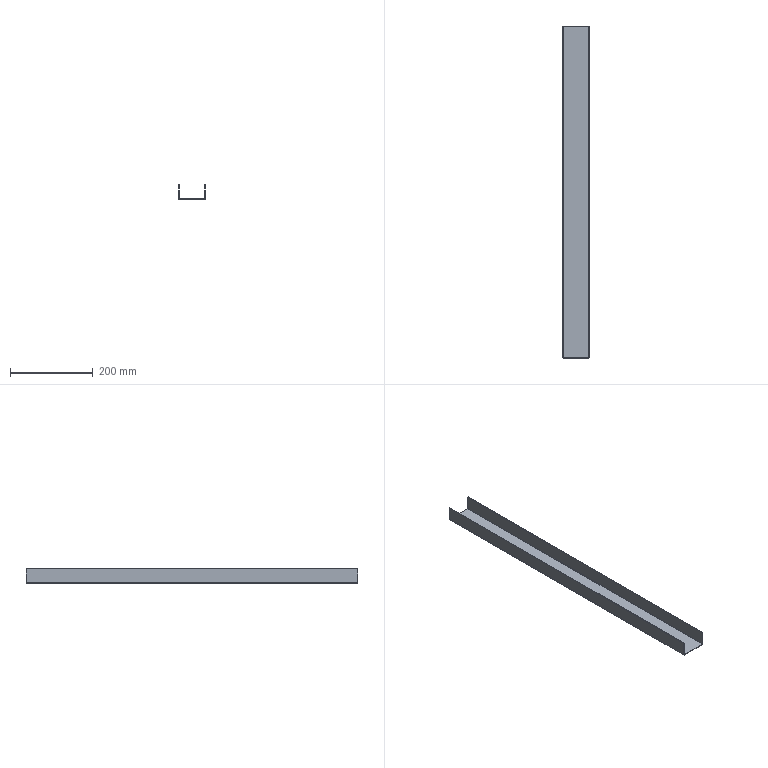Part | STEP file | Trunking Light 6 | 1 solid | 14 faces | box 65 x 800 x 35 mm | volume 157112 mm3 | plane 10 | cylinder 4 | commonest cylinder face diameters 1 x2 4 x2
STEP:
#1=CARTESIAN_POINT('',(61.399,612.395,-1.5));
#2=VERTEX_POINT('',#1);
#3=CARTESIAN_POINT('',(0.399,612.395,-1.5));
#4=VERTEX_POINT('',#3);
#5=CARTESIAN_POINT('',(0.,612.395,-1.5));
#6=DIRECTION('',(-1.,0.,0.));
#7=VECTOR('',#6,1000.);
#8=LINE('',#5,#7);
#9=EDGE_CURVE('',#2,#4,#8,.T.);
#10=ORIENTED_EDGE('',*,*,#9,.F.);
#11=CARTESIAN_POINT('',(61.399,-187.605,-1.5));
#12=VERTEX_POINT('',#11);
#13=CARTESIAN_POINT('',(61.399,0.,-1.5));
#14=DIRECTION('',(0.,1.,0.));
#15=VECTOR('',#14,1000.);
#16=LINE('',#13,#15);
#17=EDGE_CURVE('',#12,#2,#16,.T.);
#18=ORIENTED_EDGE('',*,*,#17,.F.);
#19=CARTESIAN_POINT('',(0.399,-187.605,-1.5));
#20=VERTEX_POINT('',#19);
#21=CARTESIAN_POINT('',(0.,-187.605,-1.5));
#22=DIRECTION('',(1.,0.,0.));
#23=VECTOR('',#22,1000.);
#24=LINE('',#21,#23);
#25=EDGE_CURVE('',#20,#12,#24,.T.);
#26=ORIENTED_EDGE('',*,*,#25,.F.);
#27=CARTESIAN_POINT('',(0.399,0.,-1.5));
#28=DIRECTION('',(0.,-1.,0.));
#29=VECTOR('',#28,1000.);
#30=LINE('',#27,#29);
#31=EDGE_CURVE('',#4,#20,#30,.T.);
#32=ORIENTED_EDGE('',*,*,#31,.F.);
#33=EDGE_LOOP('',(#10,#18,#26,#32));
#34=FACE_OUTER_BOUND('',#33,.T.);
#35=CARTESIAN_POINT('',(0.,0.,-1.5));
#36=DIRECTION('',(0.,0.,1.));
#37=DIRECTION('',(1.,0.,0.));
#38=AXIS2_PLACEMENT_3D('',#35,#36,#37);
#39=PLANE('',#38);
#40=ADVANCED_FACE('',(#34),#39,.F.);
#41=CARTESIAN_POINT('',(-1.601,-187.605,0.5));
#42=VERTEX_POINT('',#41);
#43=CARTESIAN_POINT('',(-1.601,612.395,0.5));
#44=VERTEX_POINT('',#43);
#45=CARTESIAN_POINT('',(-1.601,-187.605,0.5));
#46=DIRECTION('',(0.,1.,0.));
#47=VECTOR('',#46,1000.);
#48=LINE('',#45,#47);
#49=EDGE_CURVE('',#42,#44,#48,.T.);
#50=ORIENTED_EDGE('',*,*,#49,.T.);
#51=CARTESIAN_POINT('',(0.399,612.395,0.5));
#52=DIRECTION('',(0.,-1.,0.));
#53=DIRECTION('',(1.,0.,0.));
#54=AXIS2_PLACEMENT_3D('',#51,#52,#53);
#55=CIRCLE('',#54,2.);
#56=EDGE_CURVE('',#44,#4,#55,.T.);
#57=ORIENTED_EDGE('',*,*,#56,.T.);
#58=ORIENTED_EDGE('',*,*,#31,.T.);
#59=CARTESIAN_POINT('',(0.399,-187.605,0.5));
#60=DIRECTION('',(0.,1.,0.));
#61=DIRECTION('',(1.,0.,0.));
#62=AXIS2_PLACEMENT_3D('',#59,#60,#61);
#63=CIRCLE('',#62,2.);
#64=EDGE_CURVE('',#20,#42,#63,.T.);
#65=ORIENTED_EDGE('',*,*,#64,.T.);
#66=EDGE_LOOP('',(#50,#57,#58,#65));
#67=FACE_OUTER_BOUND('',#66,.T.);
#68=CARTESIAN_POINT('',(0.399,-187.605,0.5));
#69=DIRECTION('',(0.,-1.,0.));
#70=DIRECTION('',(1.,0.,0.));
#71=AXIS2_PLACEMENT_3D('',#68,#69,#70);
#72=CYLINDRICAL_SURFACE('',#71,2.);
#73=ADVANCED_FACE('',(#67),#72,.T.);
#74=CARTESIAN_POINT('',(0.399,612.395,0.));
#75=VERTEX_POINT('',#74);
#76=CARTESIAN_POINT('',(61.399,612.395,0.));
#77=VERTEX_POINT('',#76);
#78=CARTESIAN_POINT('',(-1.601,612.395,0.));
#79=DIRECTION('',(1.,0.,0.));
#80=VECTOR('',#79,1000.);
#81=LINE('',#78,#80);
#82=EDGE_CURVE('',#75,#77,#81,.T.);
#83=ORIENTED_EDGE('',*,*,#82,.T.);
#84=CARTESIAN_POINT('',(61.899,612.395,0.5));
#85=VERTEX_POINT('',#84);
#86=CARTESIAN_POINT('',(61.399,612.395,0.5));
#87=DIRECTION('',(0.,1.,0.));
#88=DIRECTION('',(0.,0.,1.));
#89=AXIS2_PLACEMENT_3D('',#86,#87,#88);
#90=CIRCLE('',#89,0.5);
#91=EDGE_CURVE('',#85,#77,#90,.T.);
#92=ORIENTED_EDGE('',*,*,#91,.F.);
#93=CARTESIAN_POINT('',(61.899,612.395,33.5));
#94=VERTEX_POINT('',#93);
#95=CARTESIAN_POINT('',(61.899,612.395,33.5));
#96=DIRECTION('',(0.,0.,-1.));
#97=VECTOR('',#96,1000.);
#98=LINE('',#95,#97);
#99=EDGE_CURVE('',#94,#85,#98,.T.);
#100=ORIENTED_EDGE('',*,*,#99,.F.);
#101=CARTESIAN_POINT('',(63.399,612.395,33.5));
#102=VERTEX_POINT('',#101);
#103=CARTESIAN_POINT('',(63.399,612.395,33.5));
#104=DIRECTION('',(-1.,0.,0.));
#105=VECTOR('',#104,1000.);
#106=LINE('',#103,#105);
#107=EDGE_CURVE('',#102,#94,#106,.T.);
#108=ORIENTED_EDGE('',*,*,#107,.F.);
#109=CARTESIAN_POINT('',(63.399,612.395,0.5));
#110=VERTEX_POINT('',#109);
#111=CARTESIAN_POINT('',(63.399,612.395,0.));
#112=DIRECTION('',(0.,0.,-1.));
#113=VECTOR('',#112,1000.);
#114=LINE('',#111,#113);
#115=EDGE_CURVE('',#102,#110,#114,.T.);
#116=ORIENTED_EDGE('',*,*,#115,.T.);
#117=CARTESIAN_POINT('',(61.399,612.395,0.5));
#118=DIRECTION('',(0.,-1.,0.));
#119=DIRECTION('',(0.,0.,1.));
#120=AXIS2_PLACEMENT_3D('',#117,#118,#119);
#121=CIRCLE('',#120,2.);
#122=EDGE_CURVE('',#2,#110,#121,.T.);
#123=ORIENTED_EDGE('',*,*,#122,.F.);
#124=ORIENTED_EDGE('',*,*,#9,.T.);
#125=ORIENTED_EDGE('',*,*,#56,.F.);
#126=CARTESIAN_POINT('',(-1.601,612.395,33.5));
#127=VERTEX_POINT('',#126);
#128=CARTESIAN_POINT('',(-1.601,612.395,0.));
#129=DIRECTION('',(0.,0.,1.));
#130=VECTOR('',#129,1000.);
#131=LINE('',#128,#130);
#132=EDGE_CURVE('',#44,#127,#131,.T.);
#133=ORIENTED_EDGE('',*,*,#132,.T.);
#134=CARTESIAN_POINT('',(-0.101,612.395,33.5));
#135=VERTEX_POINT('',#134);
#136=CARTESIAN_POINT('',(-1.601,612.395,33.5));
#137=DIRECTION('',(1.,0.,0.));
#138=VECTOR('',#137,1000.);
#139=LINE('',#136,#138);
#140=EDGE_CURVE('',#127,#135,#139,.T.);
#141=ORIENTED_EDGE('',*,*,#140,.T.);
#142=CARTESIAN_POINT('',(-0.101,612.395,0.5));
#143=VERTEX_POINT('',#142);
#144=CARTESIAN_POINT('',(-0.101,612.395,0.));
#145=DIRECTION('',(0.,0.,1.));
#146=VECTOR('',#145,1000.);
#147=LINE('',#144,#146);
#148=EDGE_CURVE('',#143,#135,#147,.T.);
#149=ORIENTED_EDGE('',*,*,#148,.F.);
#150=CARTESIAN_POINT('',(0.399,612.395,0.5));
#151=DIRECTION('',(0.,-1.,0.));
#152=DIRECTION('',(1.,0.,0.));
#153=AXIS2_PLACEMENT_3D('',#150,#151,#152);
#154=CIRCLE('',#153,0.5);
#155=EDGE_CURVE('',#143,#75,#154,.T.);
#156=ORIENTED_EDGE('',*,*,#155,.T.);
#157=EDGE_LOOP('',(#83,#92,#100,#108,#116,#123,#124,#125,#133,#141,#149,#156));
#158=FACE_OUTER_BOUND('',#157,.T.);
#159=CARTESIAN_POINT('',(-1.601,612.395,-1.5));
#160=DIRECTION('',(0.,1.,0.));
#161=DIRECTION('',(0.,0.,1.));
#162=AXIS2_PLACEMENT_3D('',#159,#160,#161);
#163=PLANE('',#162);
#164=ADVANCED_FACE('',(#158),#163,.T.);
#165=CARTESIAN_POINT('',(63.399,-187.605,0.5));
#166=VERTEX_POINT('',#165);
#167=CARTESIAN_POINT('',(63.399,612.395,0.5));
#168=DIRECTION('',(0.,-1.,0.));
#169=VECTOR('',#168,1000.);
#170=LINE('',#167,#169);
#171=EDGE_CURVE('',#110,#166,#170,.T.);
#172=ORIENTED_EDGE('',*,*,#171,.T.);
#173=CARTESIAN_POINT('',(61.399,-187.605,0.5));
#174=DIRECTION('',(0.,1.,0.));
#175=DIRECTION('',(0.,0.,1.));
#176=AXIS2_PLACEMENT_3D('',#173,#174,#175);
#177=CIRCLE('',#176,2.);
#178=EDGE_CURVE('',#166,#12,#177,.T.);
#179=ORIENTED_EDGE('',*,*,#178,.T.);
#180=ORIENTED_EDGE('',*,*,#17,.T.);
#181=ORIENTED_EDGE('',*,*,#122,.T.);
#182=EDGE_LOOP('',(#172,#179,#180,#181));
#183=FACE_OUTER_BOUND('',#182,.T.);
#184=CARTESIAN_POINT('',(61.399,612.395,0.5));
#185=DIRECTION('',(0.,1.,0.));
#186=DIRECTION('',(0.,0.,1.));
#187=AXIS2_PLACEMENT_3D('',#184,#185,#186);
#188=CYLINDRICAL_SURFACE('',#187,2.);
#189=ADVANCED_FACE('',(#183),#188,.T.);
#190=ORIENTED_EDGE('',*,*,#25,.T.);
#191=ORIENTED_EDGE('',*,*,#178,.F.);
#192=CARTESIAN_POINT('',(63.399,-187.605,33.5));
#193=VERTEX_POINT('',#192);
#194=CARTESIAN_POINT('',(63.399,-187.605,0.));
#195=DIRECTION('',(0.,0.,1.));
#196=VECTOR('',#195,1000.);
#197=LINE('',#194,#196);
#198=EDGE_CURVE('',#166,#193,#197,.T.);
#199=ORIENTED_EDGE('',*,*,#198,.T.);
#200=CARTESIAN_POINT('',(61.899,-187.605,33.5));
#201=VERTEX_POINT('',#200);
#202=CARTESIAN_POINT('',(63.399,-187.605,33.5));
#203=DIRECTION('',(-1.,0.,0.));
#204=VECTOR('',#203,1000.);
#205=LINE('',#202,#204);
#206=EDGE_CURVE('',#193,#201,#205,.T.);
#207=ORIENTED_EDGE('',*,*,#206,.T.);
#208=CARTESIAN_POINT('',(61.899,-187.605,0.5));
#209=VERTEX_POINT('',#208);
#210=CARTESIAN_POINT('',(61.899,-187.605,0.));
#211=DIRECTION('',(0.,0.,1.));
#212=VECTOR('',#211,1000.);
#213=LINE('',#210,#212);
#214=EDGE_CURVE('',#209,#201,#213,.T.);
#215=ORIENTED_EDGE('',*,*,#214,.F.);
#216=CARTESIAN_POINT('',(61.399,-187.605,0.));
#217=VERTEX_POINT('',#216);
#218=CARTESIAN_POINT('',(61.399,-187.605,0.5));
#219=DIRECTION('',(0.,1.,0.));
#220=DIRECTION('',(0.,0.,1.));
#221=AXIS2_PLACEMENT_3D('',#218,#219,#220);
#222=CIRCLE('',#221,0.5);
#223=EDGE_CURVE('',#209,#217,#222,.T.);
#224=ORIENTED_EDGE('',*,*,#223,.T.);
#225=CARTESIAN_POINT('',(0.399,-187.605,0.));
#226=VERTEX_POINT('',#225);
#227=CARTESIAN_POINT('',(-1.601,-187.605,0.));
#228=DIRECTION('',(-1.,0.,0.));
#229=VECTOR('',#228,1000.);
#230=LINE('',#227,#229);
#231=EDGE_CURVE('',#217,#226,#230,.T.);
#232=ORIENTED_EDGE('',*,*,#231,.T.);
#233=CARTESIAN_POINT('',(-0.101,-187.605,0.5));
#234=VERTEX_POINT('',#233);
#235=CARTESIAN_POINT('',(0.399,-187.605,0.5));
#236=DIRECTION('',(0.,1.,0.));
#237=DIRECTION('',(1.,0.,0.));
#238=AXIS2_PLACEMENT_3D('',#235,#236,#237);
#239=CIRCLE('',#238,0.5);
#240=EDGE_CURVE('',#226,#234,#239,.T.);
#241=ORIENTED_EDGE('',*,*,#240,.T.);
#242=CARTESIAN_POINT('',(-0.101,-187.605,33.5));
#243=VERTEX_POINT('',#242);
#244=CARTESIAN_POINT('',(-0.101,-187.605,33.5));
#245=DIRECTION('',(0.,0.,-1.));
#246=VECTOR('',#245,1000.);
#247=LINE('',#244,#246);
#248=EDGE_CURVE('',#243,#234,#247,.T.);
#249=ORIENTED_EDGE('',*,*,#248,.F.);
#250=CARTESIAN_POINT('',(-1.601,-187.605,33.5));
#251=VERTEX_POINT('',#250);
#252=CARTESIAN_POINT('',(-1.601,-187.605,33.5));
#253=DIRECTION('',(1.,0.,0.));
#254=VECTOR('',#253,1000.);
#255=LINE('',#252,#254);
#256=EDGE_CURVE('',#251,#243,#255,.T.);
#257=ORIENTED_EDGE('',*,*,#256,.F.);
#258=CARTESIAN_POINT('',(-1.601,-187.605,0.));
#259=DIRECTION('',(0.,0.,-1.));
#260=VECTOR('',#259,1000.);
#261=LINE('',#258,#260);
#262=EDGE_CURVE('',#251,#42,#261,.T.);
#263=ORIENTED_EDGE('',*,*,#262,.T.);
#264=ORIENTED_EDGE('',*,*,#64,.F.);
#265=EDGE_LOOP('',(#190,#191,#199,#207,#215,#224,#232,#241,#249,#257,#263,#264));
#266=FACE_OUTER_BOUND('',#265,.T.);
#267=CARTESIAN_POINT('',(-1.601,-187.605,-1.5));
#268=DIRECTION('',(0.,-1.,0.));
#269=DIRECTION('',(0.,0.,-1.));
#270=AXIS2_PLACEMENT_3D('',#267,#268,#269);
#271=PLANE('',#270);
#272=ADVANCED_FACE('',(#266),#271,.T.);
#273=ORIENTED_EDGE('',*,*,#262,.F.);
#274=CARTESIAN_POINT('',(-1.601,0.,33.5));
#275=DIRECTION('',(0.,-1.,0.));
#276=VECTOR('',#275,1000.);
#277=LINE('',#274,#276);
#278=EDGE_CURVE('',#127,#251,#277,.T.);
#279=ORIENTED_EDGE('',*,*,#278,.F.);
#280=ORIENTED_EDGE('',*,*,#132,.F.);
#281=ORIENTED_EDGE('',*,*,#49,.F.);
#282=EDGE_LOOP('',(#273,#279,#280,#281));
#283=FACE_OUTER_BOUND('',#282,.T.);
#284=CARTESIAN_POINT('',(-1.601,0.,0.));
#285=DIRECTION('',(1.,0.,0.));
#286=DIRECTION('',(0.,0.,-1.));
#287=AXIS2_PLACEMENT_3D('',#284,#285,#286);
#288=PLANE('',#287);
#289=ADVANCED_FACE('',(#283),#288,.F.);
#290=ORIENTED_EDGE('',*,*,#231,.F.);
#291=CARTESIAN_POINT('',(61.399,0.,0.));
#292=DIRECTION('',(0.,1.,0.));
#293=VECTOR('',#292,1000.);
#294=LINE('',#291,#293);
#295=EDGE_CURVE('',#217,#77,#294,.T.);
#296=ORIENTED_EDGE('',*,*,#295,.T.);
#297=ORIENTED_EDGE('',*,*,#82,.F.);
#298=CARTESIAN_POINT('',(0.399,0.,0.));
#299=DIRECTION('',(0.,-1.,0.));
#300=VECTOR('',#299,1000.);
#301=LINE('',#298,#300);
#302=EDGE_CURVE('',#75,#226,#301,.T.);
#303=ORIENTED_EDGE('',*,*,#302,.T.);
#304=EDGE_LOOP('',(#290,#296,#297,#303));
#305=FACE_OUTER_BOUND('',#304,.T.);
#306=CARTESIAN_POINT('',(0.,0.,0.));
#307=DIRECTION('',(0.,0.,1.));
#308=DIRECTION('',(1.,0.,0.));
#309=AXIS2_PLACEMENT_3D('',#306,#307,#308);
#310=PLANE('',#309);
#311=ADVANCED_FACE('',(#305),#310,.T.);
#312=ORIENTED_EDGE('',*,*,#115,.F.);
#313=CARTESIAN_POINT('',(63.399,0.,33.5));
#314=DIRECTION('',(0.,1.,0.));
#315=VECTOR('',#314,1000.);
#316=LINE('',#313,#315);
#317=EDGE_CURVE('',#193,#102,#316,.T.);
#318=ORIENTED_EDGE('',*,*,#317,.F.);
#319=ORIENTED_EDGE('',*,*,#198,.F.);
#320=ORIENTED_EDGE('',*,*,#171,.F.);
#321=EDGE_LOOP('',(#312,#318,#319,#320));
#322=FACE_OUTER_BOUND('',#321,.T.);
#323=CARTESIAN_POINT('',(63.399,0.,0.));
#324=DIRECTION('',(-1.,0.,0.));
#325=DIRECTION('',(0.,0.,1.));
#326=AXIS2_PLACEMENT_3D('',#323,#324,#325);
#327=PLANE('',#326);
#328=ADVANCED_FACE('',(#322),#327,.F.);
#329=ORIENTED_EDGE('',*,*,#140,.F.);
#330=ORIENTED_EDGE('',*,*,#278,.T.);
#331=ORIENTED_EDGE('',*,*,#256,.T.);
#332=CARTESIAN_POINT('',(-0.101,612.395,33.5));
#333=DIRECTION('',(0.,-1.,0.));
#334=VECTOR('',#333,1000.);
#335=LINE('',#332,#334);
#336=EDGE_CURVE('',#135,#243,#335,.T.);
#337=ORIENTED_EDGE('',*,*,#336,.F.);
#338=EDGE_LOOP('',(#329,#330,#331,#337));
#339=FACE_OUTER_BOUND('',#338,.T.);
#340=CARTESIAN_POINT('',(-1.601,612.395,33.5));
#341=DIRECTION('',(0.,0.,-1.));
#342=DIRECTION('',(-1.,0.,0.));
#343=AXIS2_PLACEMENT_3D('',#340,#341,#342);
#344=PLANE('',#343);
#345=ADVANCED_FACE('',(#339),#344,.F.);
#346=ORIENTED_EDGE('',*,*,#223,.F.);
#347=CARTESIAN_POINT('',(61.899,612.395,0.5));
#348=DIRECTION('',(0.,-1.,0.));
#349=VECTOR('',#348,1000.);
#350=LINE('',#347,#349);
#351=EDGE_CURVE('',#85,#209,#350,.T.);
#352=ORIENTED_EDGE('',*,*,#351,.F.);
#353=ORIENTED_EDGE('',*,*,#91,.T.);
#354=ORIENTED_EDGE('',*,*,#295,.F.);
#355=EDGE_LOOP('',(#346,#352,#353,#354));
#356=FACE_OUTER_BOUND('',#355,.T.);
#357=CARTESIAN_POINT('',(61.399,612.395,0.5));
#358=DIRECTION('',(0.,1.,0.));
#359=DIRECTION('',(0.,0.,1.));
#360=AXIS2_PLACEMENT_3D('',#357,#358,#359);
#361=CYLINDRICAL_SURFACE('',#360,0.5);
#362=ADVANCED_FACE('',(#356),#361,.F.);
#363=ORIENTED_EDGE('',*,*,#155,.F.);
#364=CARTESIAN_POINT('',(-0.101,-187.605,0.5));
#365=DIRECTION('',(0.,1.,0.));
#366=VECTOR('',#365,1000.);
#367=LINE('',#364,#366);
#368=EDGE_CURVE('',#234,#143,#367,.T.);
#369=ORIENTED_EDGE('',*,*,#368,.F.);
#370=ORIENTED_EDGE('',*,*,#240,.F.);
#371=ORIENTED_EDGE('',*,*,#302,.F.);
#372=EDGE_LOOP('',(#363,#369,#370,#371));
#373=FACE_OUTER_BOUND('',#372,.T.);
#374=CARTESIAN_POINT('',(0.399,-187.605,0.5));
#375=DIRECTION('',(0.,-1.,0.));
#376=DIRECTION('',(1.,0.,0.));
#377=AXIS2_PLACEMENT_3D('',#374,#375,#376);
#378=CYLINDRICAL_SURFACE('',#377,0.5);
#379=ADVANCED_FACE('',(#373),#378,.F.);
#380=ORIENTED_EDGE('',*,*,#206,.F.);
#381=ORIENTED_EDGE('',*,*,#317,.T.);
#382=ORIENTED_EDGE('',*,*,#107,.T.);
#383=CARTESIAN_POINT('',(61.899,-187.605,33.5));
#384=DIRECTION('',(0.,1.,0.));
#385=VECTOR('',#384,1000.);
#386=LINE('',#383,#385);
#387=EDGE_CURVE('',#201,#94,#386,.T.);
#388=ORIENTED_EDGE('',*,*,#387,.F.);
#389=EDGE_LOOP('',(#380,#381,#382,#388));
#390=FACE_OUTER_BOUND('',#389,.T.);
#391=CARTESIAN_POINT('',(63.399,-187.605,33.5));
#392=DIRECTION('',(0.,0.,-1.));
#393=DIRECTION('',(-1.,0.,0.));
#394=AXIS2_PLACEMENT_3D('',#391,#392,#393);
#395=PLANE('',#394);
#396=ADVANCED_FACE('',(#390),#395,.F.);
#397=ORIENTED_EDGE('',*,*,#148,.T.);
#398=ORIENTED_EDGE('',*,*,#336,.T.);
#399=ORIENTED_EDGE('',*,*,#248,.T.);
#400=ORIENTED_EDGE('',*,*,#368,.T.);
#401=EDGE_LOOP('',(#397,#398,#399,#400));
#402=FACE_OUTER_BOUND('',#401,.T.);
#403=CARTESIAN_POINT('',(-0.101,0.,0.));
#404=DIRECTION('',(1.,0.,0.));
#405=DIRECTION('',(0.,0.,-1.));
#406=AXIS2_PLACEMENT_3D('',#403,#404,#405);
#407=PLANE('',#406);
#408=ADVANCED_FACE('',(#402),#407,.T.);
#409=ORIENTED_EDGE('',*,*,#214,.T.);
#410=ORIENTED_EDGE('',*,*,#387,.T.);
#411=ORIENTED_EDGE('',*,*,#99,.T.);
#412=ORIENTED_EDGE('',*,*,#351,.T.);
#413=EDGE_LOOP('',(#409,#410,#411,#412));
#414=FACE_OUTER_BOUND('',#413,.T.);
#415=CARTESIAN_POINT('',(61.899,0.,0.));
#416=DIRECTION('',(-1.,0.,0.));
#417=DIRECTION('',(0.,0.,1.));
#418=AXIS2_PLACEMENT_3D('',#415,#416,#417);
#419=PLANE('',#418);
#420=ADVANCED_FACE('',(#414),#419,.T.);
#421=CLOSED_SHELL('',(#40,#73,#164,#189,#272,#289,#311,#328,#345,#362,#379,#396,#408,#420));
#422=MANIFOLD_SOLID_BREP('',#421);
#423=CARTESIAN_POINT('',(0.,0.,0.));
#424=DIRECTION('',(0.,0.,1.));
#425=DIRECTION('',(1.,0.,0.));
#426=AXIS2_PLACEMENT_3D('',#423,#424,#425);
#427=(LENGTH_UNIT()NAMED_UNIT(*)SI_UNIT(.MILLI.,.METRE.));
#428=UNCERTAINTY_MEASURE_WITH_UNIT(LENGTH_MEASURE(0.00001),#427,'','');
#429=(NAMED_UNIT(*)PLANE_ANGLE_UNIT()SI_UNIT($,.RADIAN.));
#430=(NAMED_UNIT(*)SI_UNIT($,.STERADIAN.)SOLID_ANGLE_UNIT());
#431=(GEOMETRIC_REPRESENTATION_CONTEXT(3)GLOBAL_UNCERTAINTY_ASSIGNED_CONTEXT((#428))GLOBAL_UNIT_ASSIGNED_CONTEXT((#427,#429,#430))REPRESENTATION_CONTEXT('',''));
#432=ADVANCED_BREP_SHAPE_REPRESENTATION('',(#422,#426),#431);